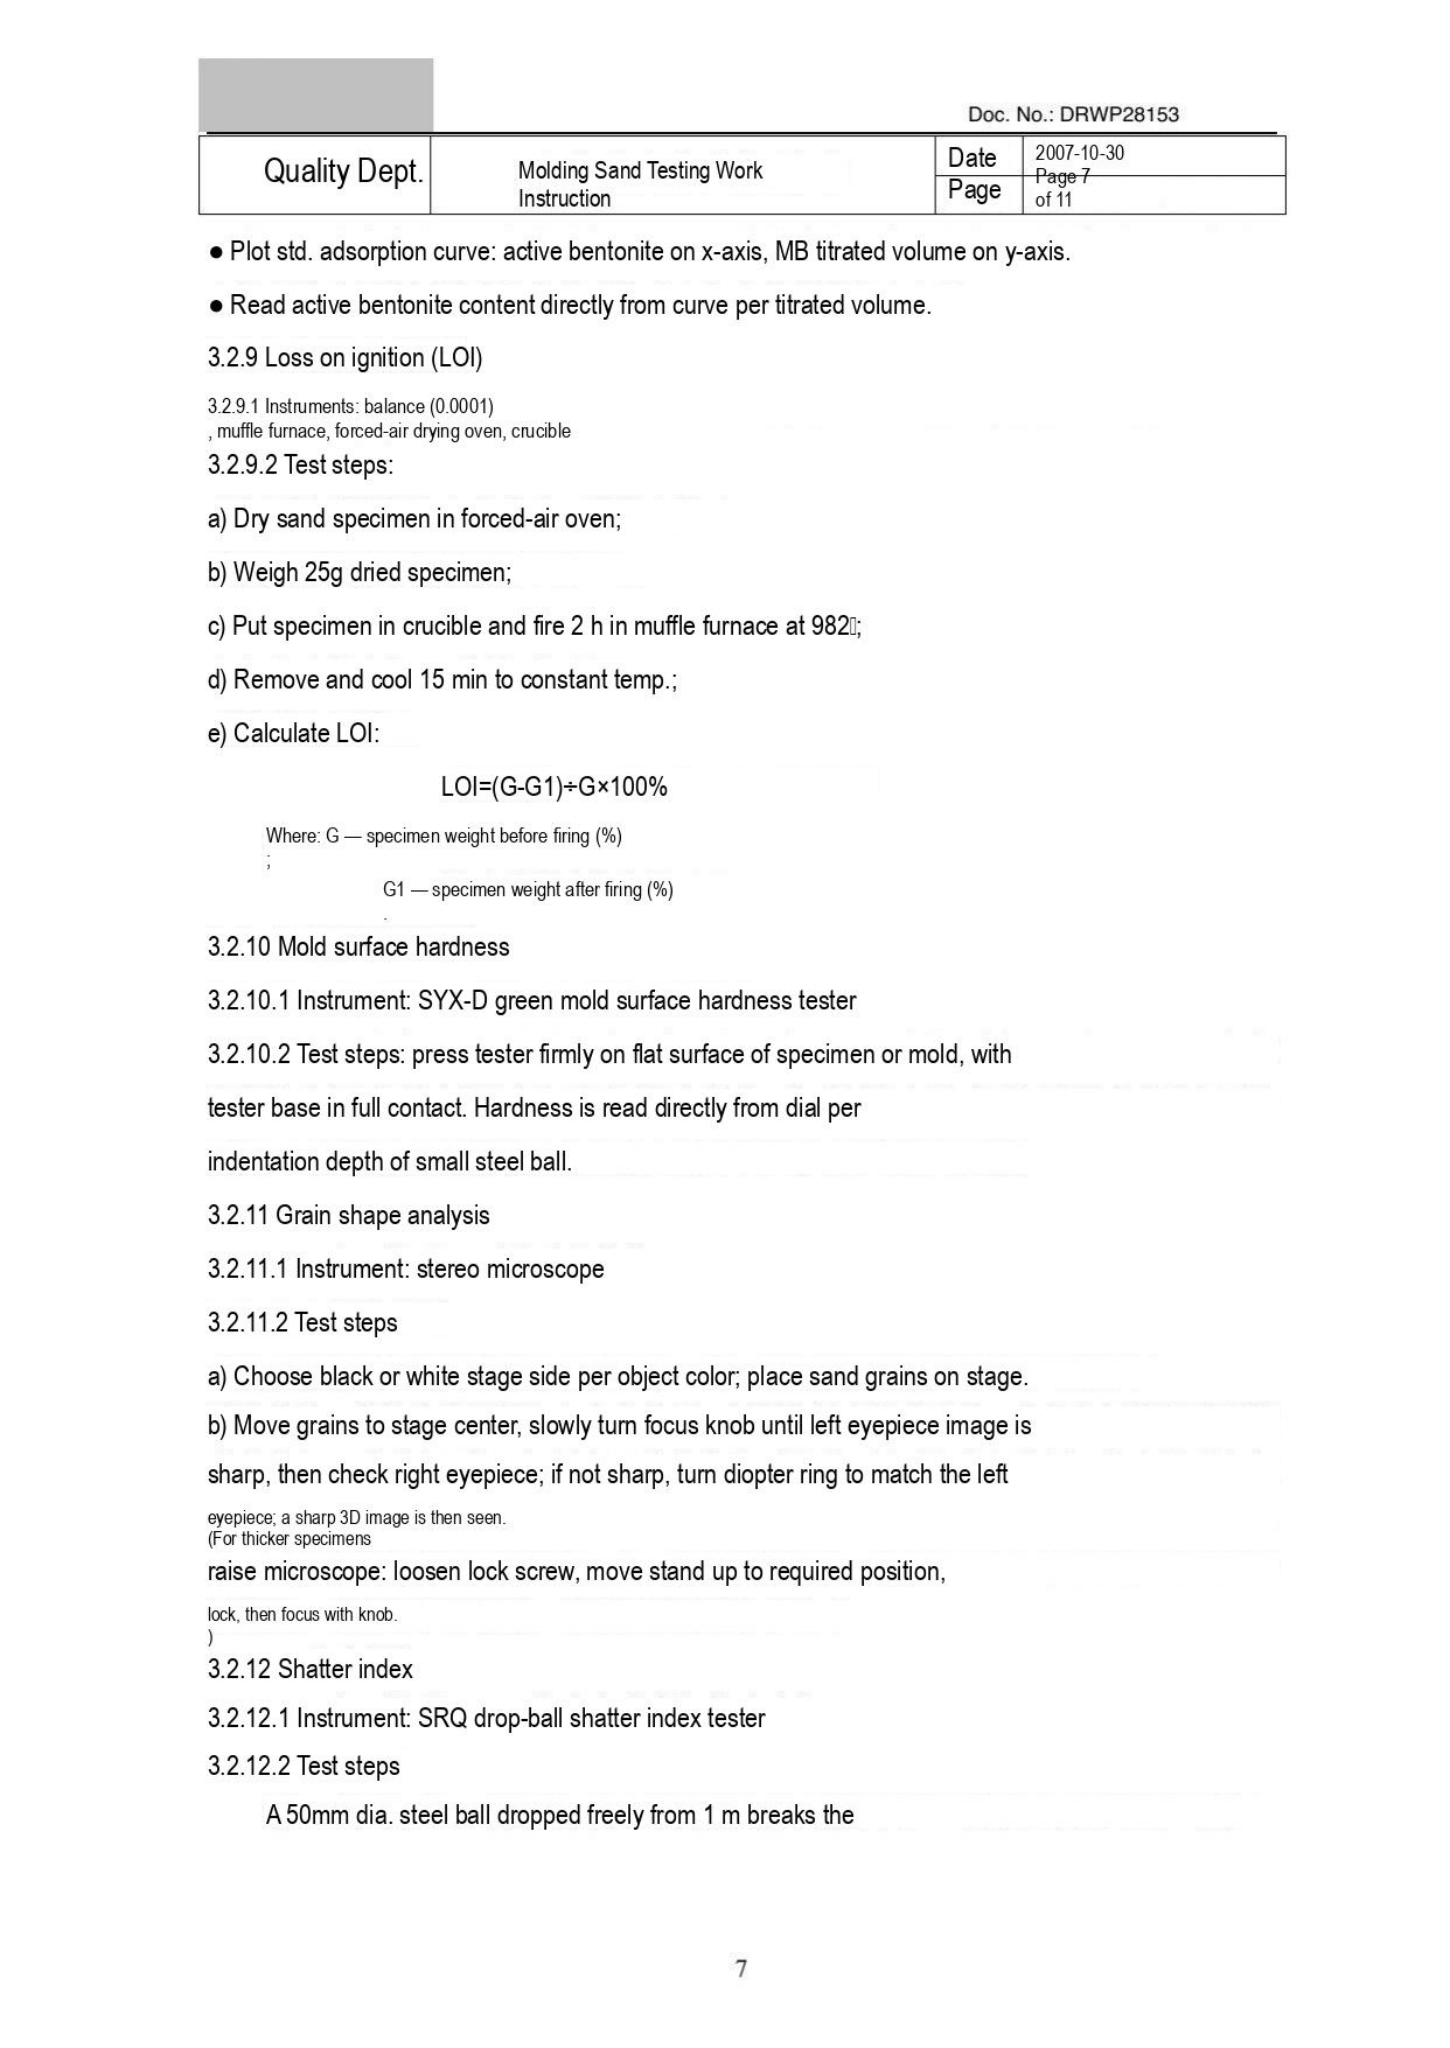Doc. No.: DRWP28153

| Quality Dept. | Molding Sand Testing Work Instruction | Date | 2007-10-30 |
|---|---|---|---|
| | | Page | Page 7 of 11 |

● Plot std. adsorption curve: active bentonite on x-axis, MB titrated volume on y-axis.

● Read active bentonite content directly from curve per titrated volume.

3.2.9 Loss on ignition (LOI)

3.2.9.1 Instruments: balance (0.0001)
, muffle furnace, forced-air drying oven, crucible

3.2.9.2 Test steps:

a) Dry sand specimen in forced-air oven;

b) Weigh 25g dried specimen;

c) Put specimen in crucible and fire 2 h in muffle furnace at 982;

d) Remove and cool 15 min to constant temp.;

e) Calculate LOI:

LOI=(G-G1)÷G×100%

Where: G — specimen weight before firing (%)
;
G1 — specimen weight after firing (%)
.

3.2.10 Mold surface hardness

3.2.10.1 Instrument: SYX-D green mold surface hardness tester

3.2.10.2 Test steps: press tester firmly on flat surface of specimen or mold, with tester base in full contact. Hardness is read directly from dial per indentation depth of small steel ball.

3.2.11 Grain shape analysis

3.2.11.1 Instrument: stereo microscope

3.2.11.2 Test steps

a) Choose black or white stage side per object color; place sand grains on stage.

b) Move grains to stage center, slowly turn focus knob until left eyepiece image is sharp, then check right eyepiece; if not sharp, turn diopter ring to match the left eyepiece; a sharp 3D image is then seen.
(For thicker specimens raise microscope: loosen lock screw, move stand up to required position, lock, then focus with knob.
)

3.2.12 Shatter index

3.2.12.1 Instrument: SRQ drop-ball shatter index tester

3.2.12.2 Test steps

A 50mm dia. steel ball dropped freely from 1 m breaks the

7
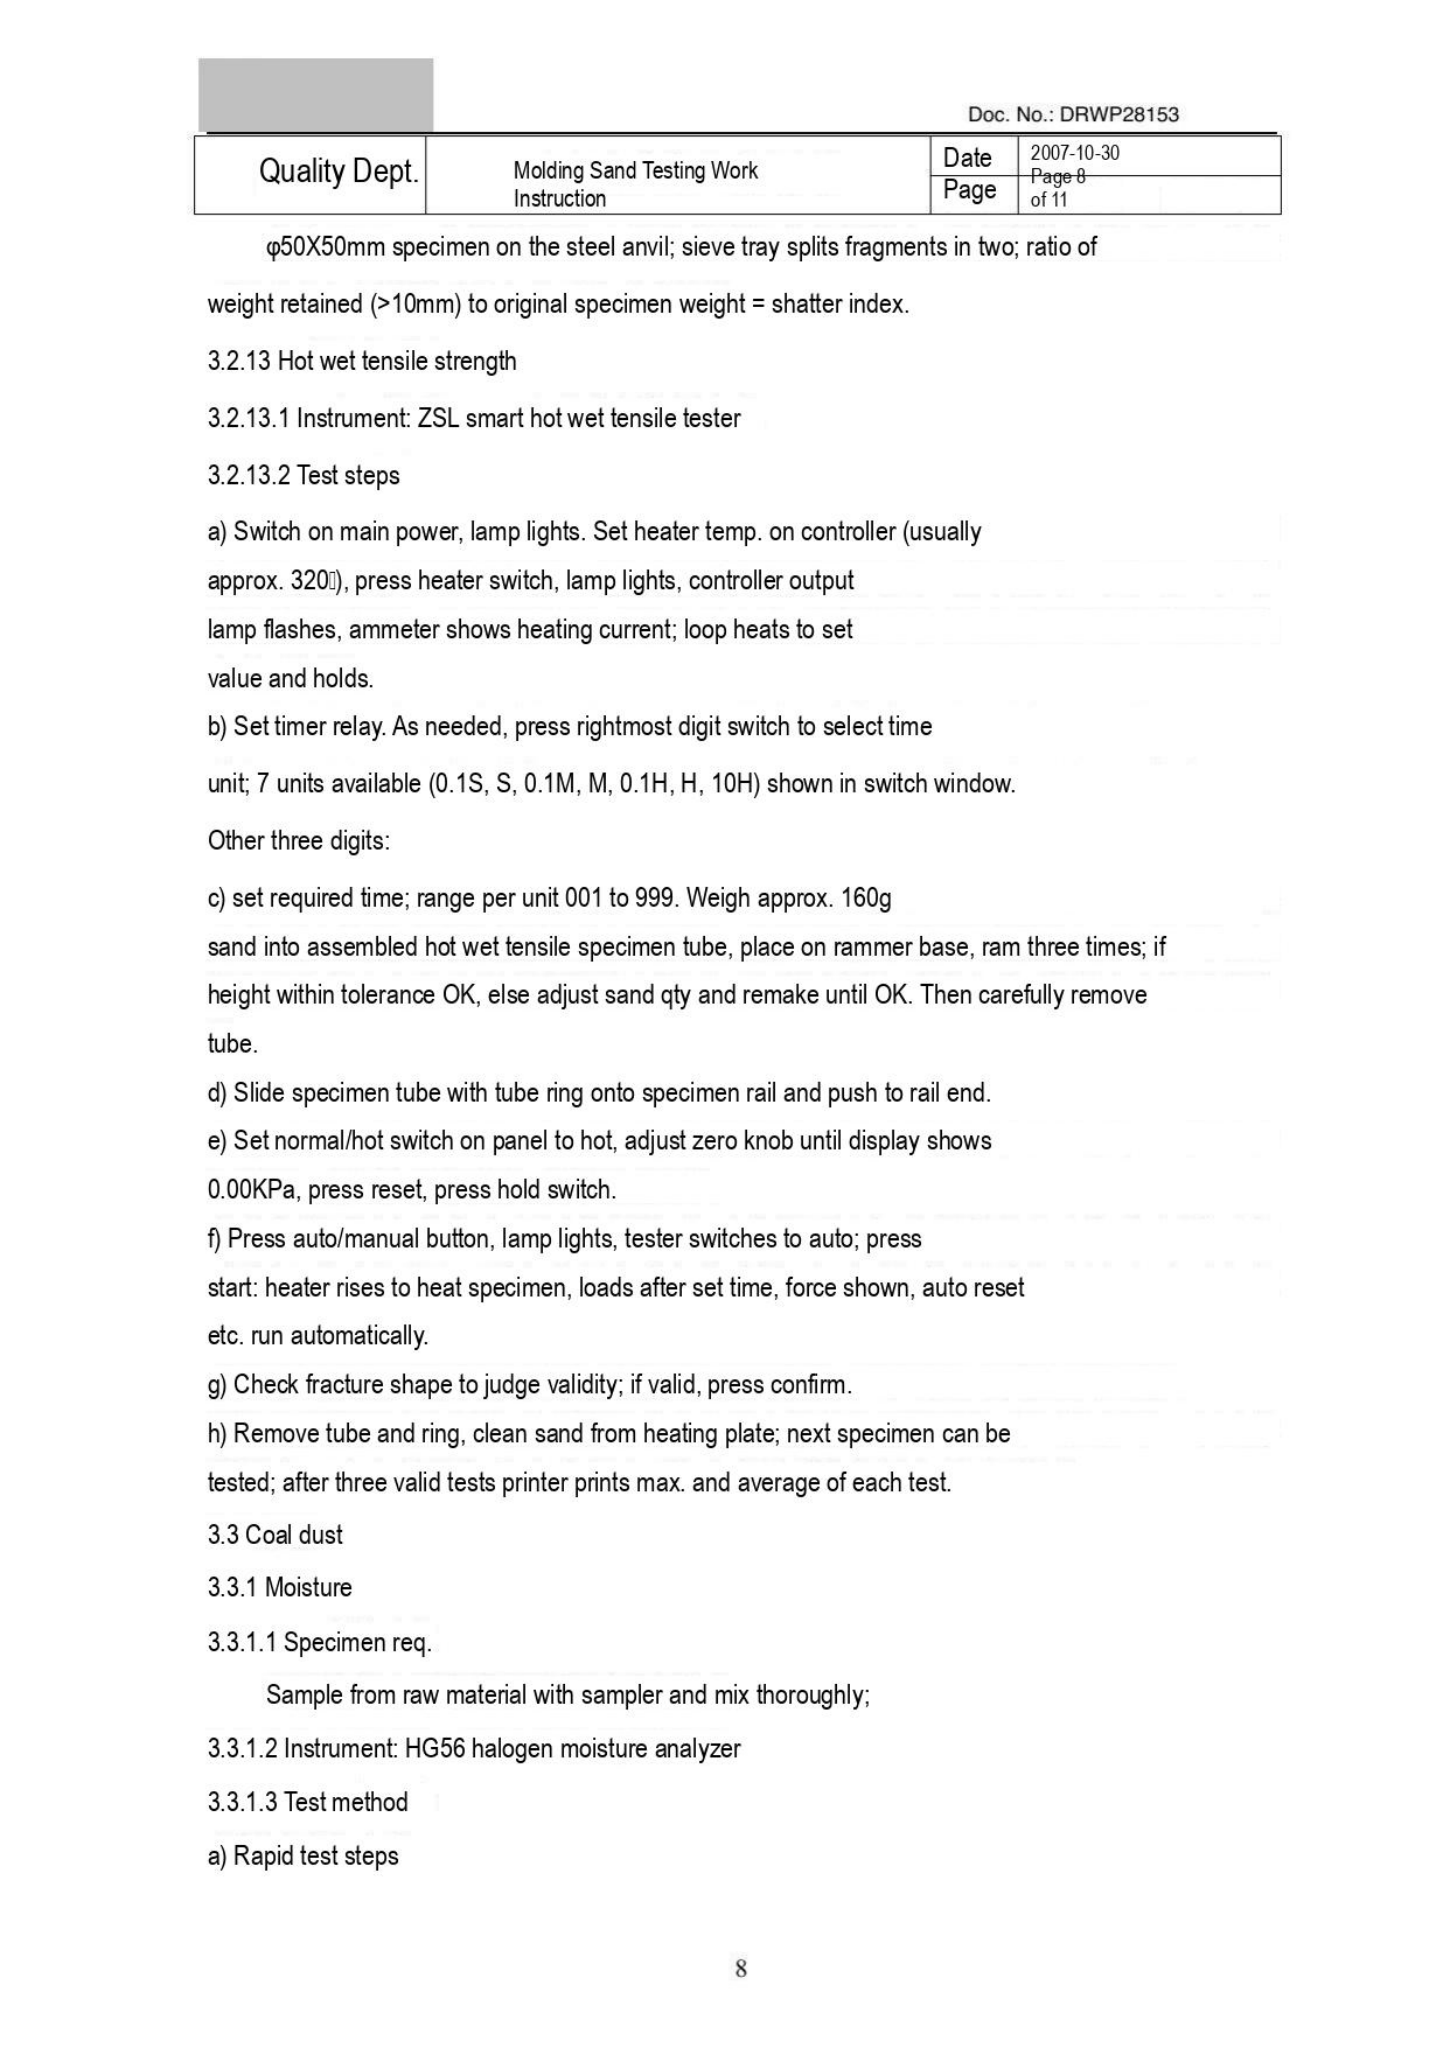Doc. No.: DRWP28153

| Quality Dept. | Molding Sand Testing Work Instruction | Date | 2007-10-30 |
|---|---|---|---|
| | | Page | Page 8 of 11 |

φ50X50mm specimen on the steel anvil; sieve tray splits fragments in two; ratio of weight retained (>10mm) to original specimen weight = shatter index.

3.2.13 Hot wet tensile strength

3.2.13.1 Instrument: ZSL smart hot wet tensile tester

3.2.13.2 Test steps

a) Switch on main power, lamp lights. Set heater temp. on controller (usually approx. 320), press heater switch, lamp lights, controller output lamp flashes, ammeter shows heating current; loop heats to set value and holds.

b) Set timer relay. As needed, press rightmost digit switch to select time unit; 7 units available (0.1S, S, 0.1M, M, 0.1H, H, 10H) shown in switch window.

Other three digits:

c) set required time; range per unit 001 to 999. Weigh approx. 160g sand into assembled hot wet tensile specimen tube, place on rammer base, ram three times; if height within tolerance OK, else adjust sand qty and remake until OK. Then carefully remove tube.

d) Slide specimen tube with tube ring onto specimen rail and push to rail end.

e) Set normal/hot switch on panel to hot, adjust zero knob until display shows 0.00KPa, press reset, press hold switch.

f) Press auto/manual button, lamp lights, tester switches to auto; press start: heater rises to heat specimen, loads after set time, force shown, auto reset etc. run automatically.

g) Check fracture shape to judge validity; if valid, press confirm.

h) Remove tube and ring, clean sand from heating plate; next specimen can be tested; after three valid tests printer prints max. and average of each test.

3.3 Coal dust

3.3.1 Moisture

3.3.1.1 Specimen req.

Sample from raw material with sampler and mix thoroughly;

3.3.1.2 Instrument: HG56 halogen moisture analyzer

3.3.1.3 Test method

a) Rapid test steps

8
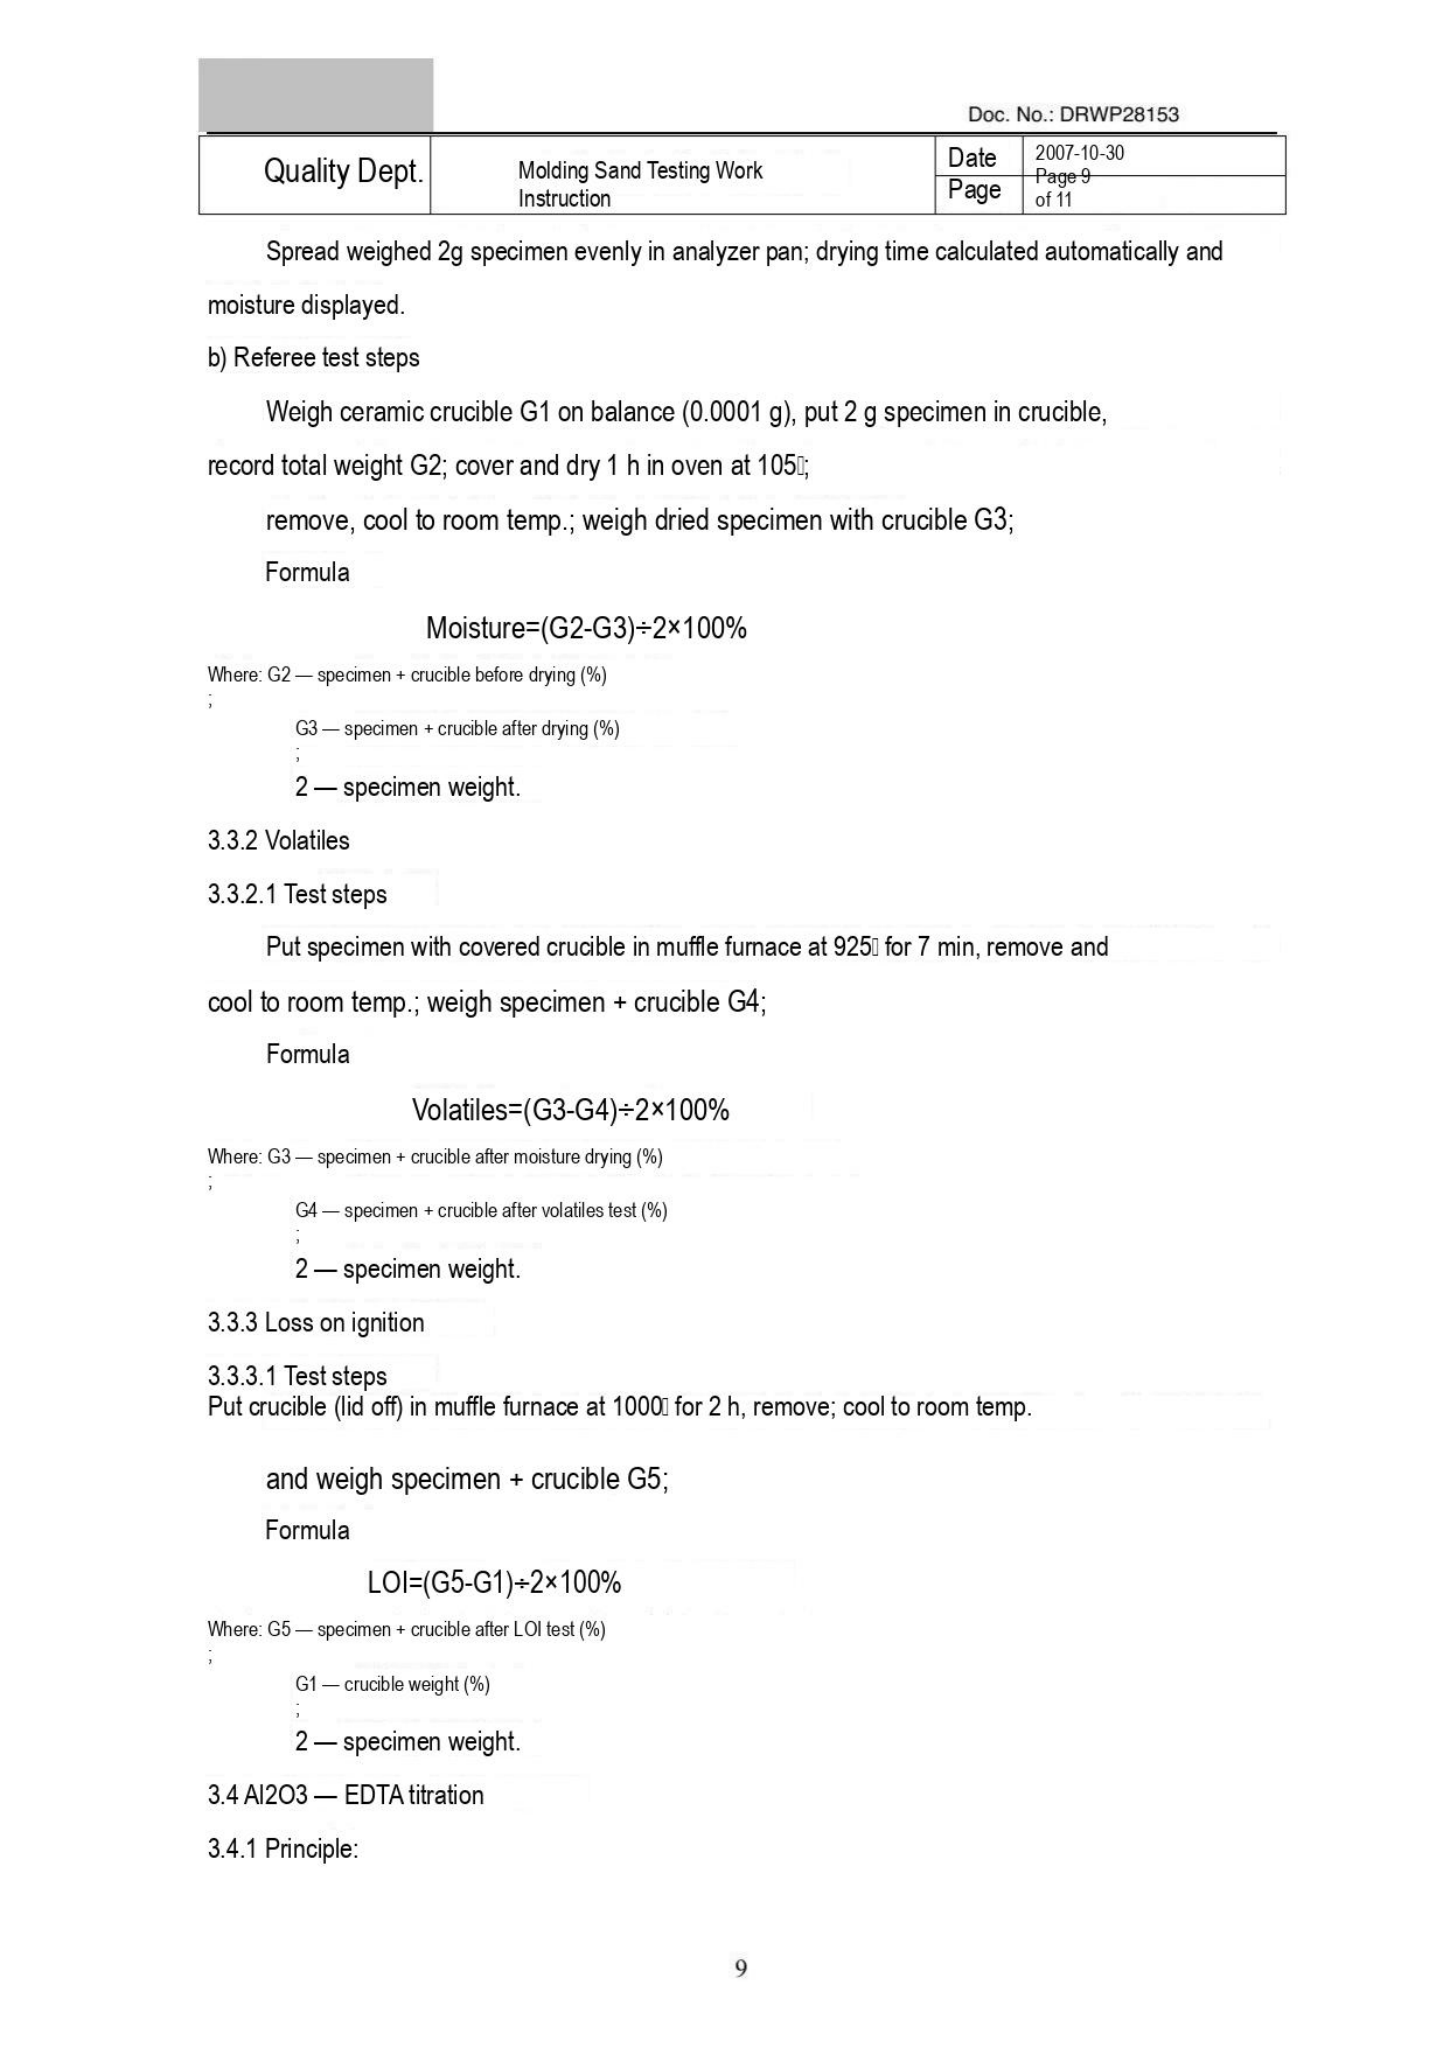Doc. No.: DRWP28153

| Quality Dept. | Molding Sand Testing Work Instruction | Date | 2007-10-30 |
|---|---|---|---|
| | | Page | Page 9 of 11 |

Spread weighed 2g specimen evenly in analyzer pan; drying time calculated automatically and moisture displayed.

b) Referee test steps

Weigh ceramic crucible G1 on balance (0.0001 g), put 2 g specimen in crucible, record total weight G2; cover and dry 1 h in oven at 105;

remove, cool to room temp.; weigh dried specimen with crucible G3;

Formula

Moisture=(G2-G3)÷2×100%

Where: G2 — specimen + crucible before drying (%)
;

G3 — specimen + crucible after drying (%)
;

2 — specimen weight.

3.3.2 Volatiles

3.3.2.1 Test steps

Put specimen with covered crucible in muffle furnace at 925 for 7 min, remove and cool to room temp.; weigh specimen + crucible G4;

Formula

Volatiles=(G3-G4)÷2×100%

Where: G3 — specimen + crucible after moisture drying (%)
;

G4 — specimen + crucible after volatiles test (%)
;

2 — specimen weight.

3.3.3 Loss on ignition

3.3.3.1 Test steps
Put crucible (lid off) in muffle furnace at 1000 for 2 h, remove; cool to room temp.

and weigh specimen + crucible G5;

Formula

LOI=(G5-G1)÷2×100%

Where: G5 — specimen + crucible after LOI test (%)
;

G1 — crucible weight (%)
;

2 — specimen weight.

3.4 Al2O3 — EDTA titration

3.4.1 Principle:

9
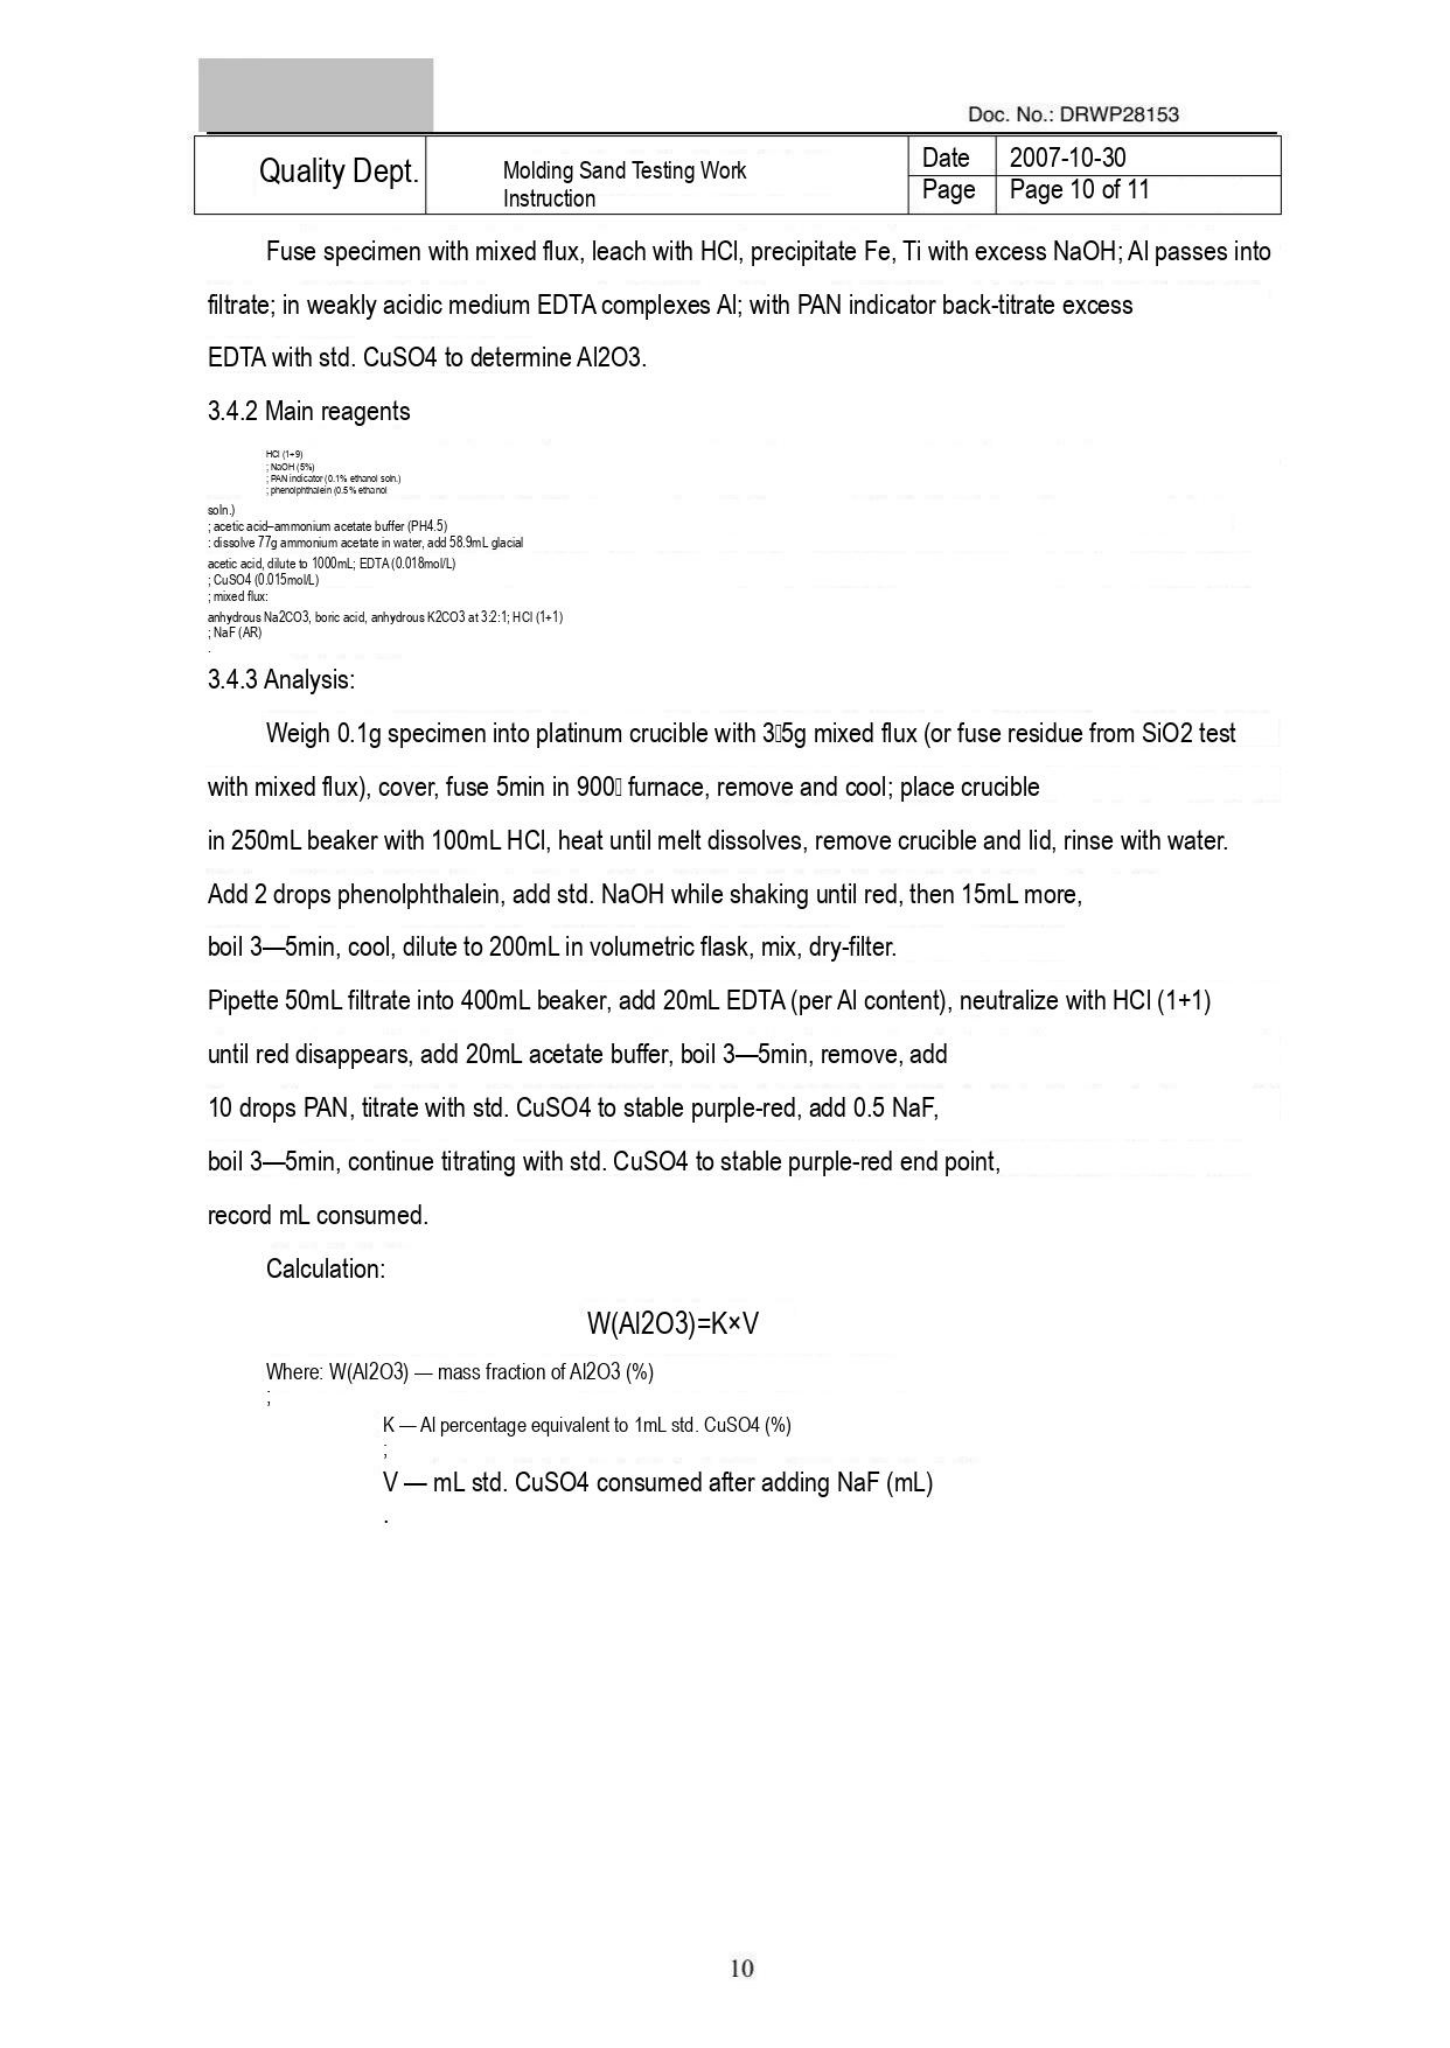Doc. No.: DRWP28153

| Quality Dept. | Molding Sand Testing Work Instruction | Date | 2007-10-30 |
|---|---|---|---|
| | | Page | Page 10 of 11 |

Fuse specimen with mixed flux, leach with HCl, precipitate Fe, Ti with excess NaOH; Al passes into filtrate; in weakly acidic medium EDTA complexes Al; with PAN indicator back-titrate excess EDTA with std. CuSO4 to determine Al2O3.

3.4.2 Main reagents

HCl (1+9)
; NaOH (5%)
; PAN indicator (0.1% ethanol soln.)
; phenolphthalein (0.5% ethanol soln.)
; acetic acid–ammonium acetate buffer (PH4.5)
: dissolve 77g ammonium acetate in water, add 58.9mL glacial acetic acid, dilute to 1000mL; EDTA (0.018mol/L)
; CuSO4 (0.015mol/L)
; mixed flux:
anhydrous Na2CO3, boric acid, anhydrous K2CO3 at 3:2:1; HCl (1+1)
; NaF (AR)
.

3.4.3 Analysis:

Weigh 0.1g specimen into platinum crucible with 3 5g mixed flux (or fuse residue from SiO2 test with mixed flux), cover, fuse 5min in 900 furnace, remove and cool; place crucible in 250mL beaker with 100mL HCl, heat until melt dissolves, remove crucible and lid, rinse with water. Add 2 drops phenolphthalein, add std. NaOH while shaking until red, then 15mL more, boil 3—5min, cool, dilute to 200mL in volumetric flask, mix, dry-filter.
Pipette 50mL filtrate into 400mL beaker, add 20mL EDTA (per Al content), neutralize with HCl (1+1) until red disappears, add 20mL acetate buffer, boil 3—5min, remove, add 10 drops PAN, titrate with std. CuSO4 to stable purple-red, add 0.5 NaF, boil 3—5min, continue titrating with std. CuSO4 to stable purple-red end point, record mL consumed.

Calculation:

W(Al2O3)=K×V

Where: W(Al2O3) — mass fraction of Al2O3 (%)
;
K — Al percentage equivalent to 1mL std. CuSO4 (%)
;
V — mL std. CuSO4 consumed after adding NaF (mL)
.

10
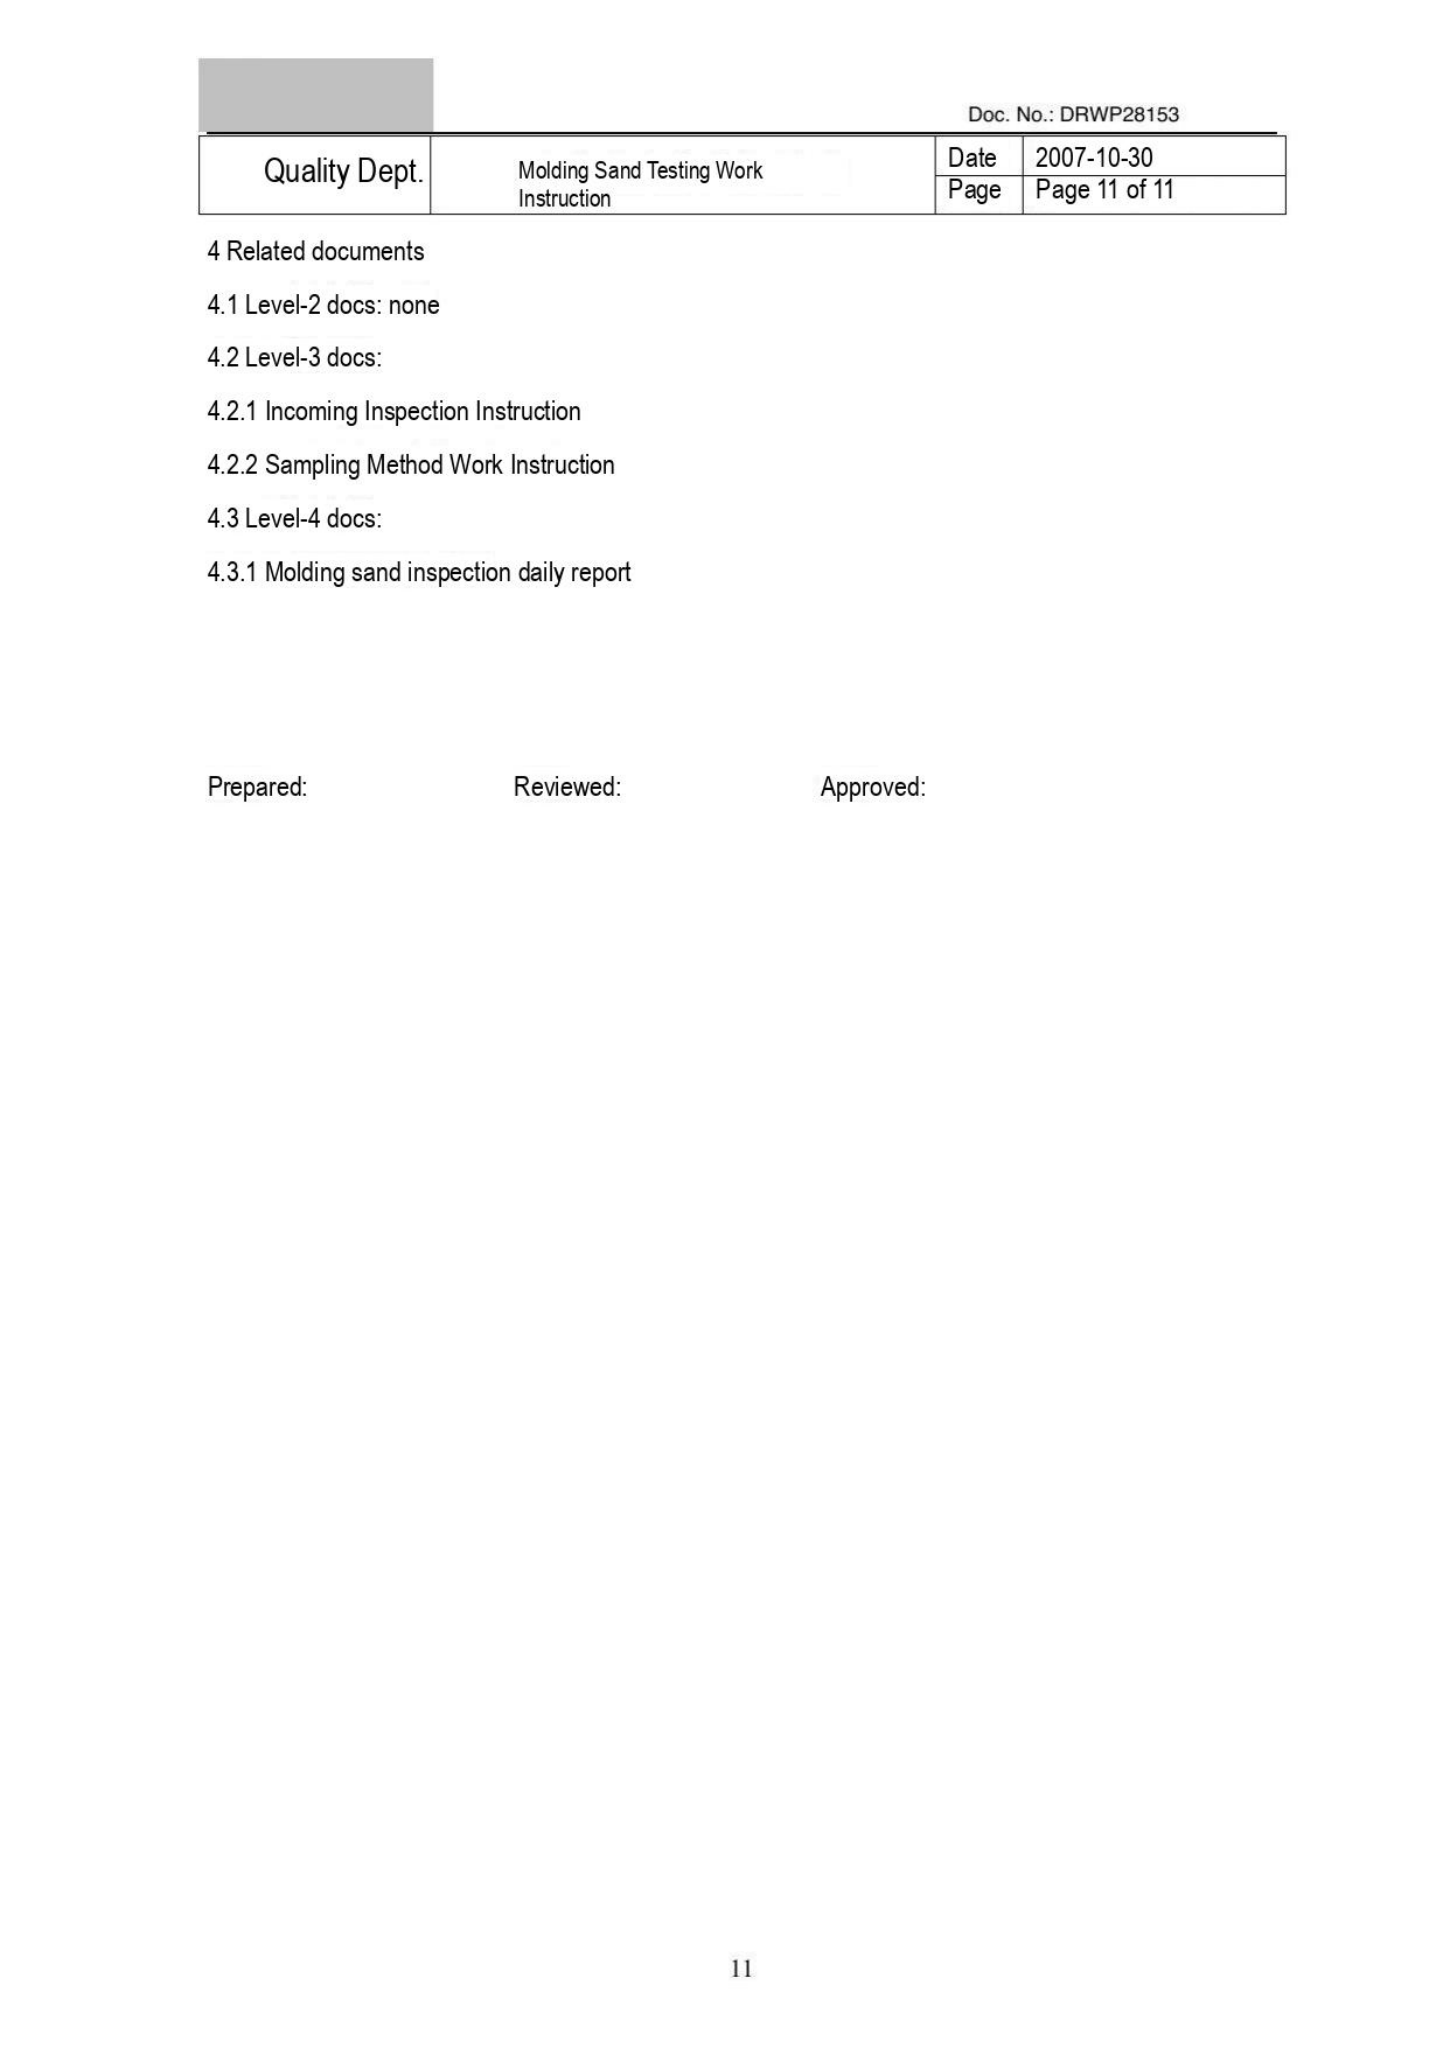Doc. No.: DRWP28153

| Quality Dept. | Molding Sand Testing Work Instruction | Date | 2007-10-30 |
|---|---|---|---|
| | | Page | Page 11 of 11 |

4 Related documents

4.1 Level-2 docs: none

4.2 Level-3 docs:

4.2.1 Incoming Inspection Instruction

4.2.2 Sampling Method Work Instruction

4.3 Level-4 docs:

4.3.1 Molding sand inspection daily report

Prepared: Reviewed: Approved:

11